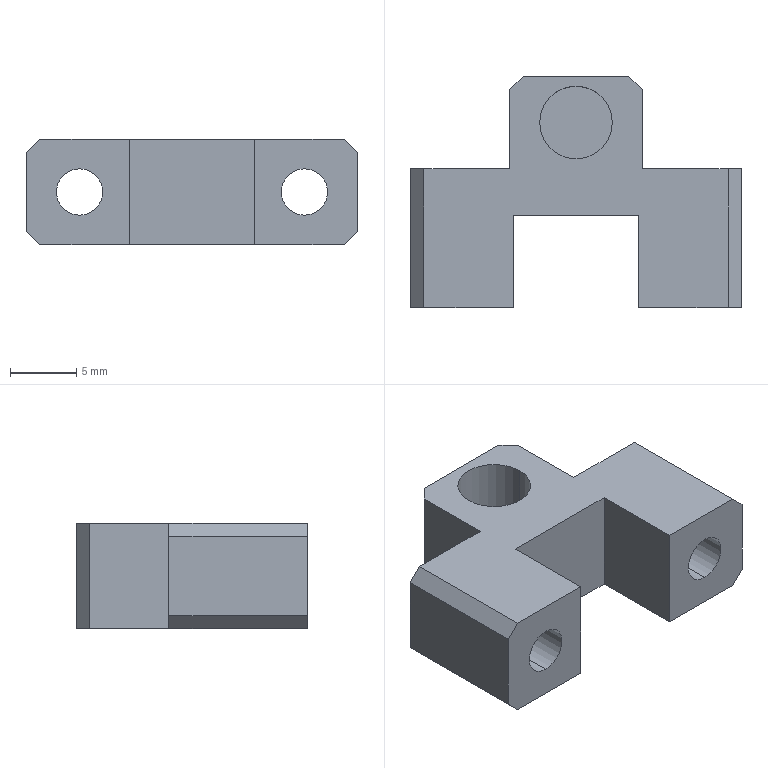Part | SolidWorks | features ICE 3, Chamfer 1, Extrusion 1, HoleWzd 1 | 1 solid | 27 faces | box 25 x 17.5 x 8 mm | volume 1778 mm3 | plane 21 | cylinder 6 | commonest cylinder face diameters 3.5 x4 5.5 x2
STEP:
#1=CARTESIAN_POINT('',(-8.5,-8.75,2.25));
#2=VERTEX_POINT('',#1);
#3=CARTESIAN_POINT('',(-8.5,-8.75,5.75));
#4=VERTEX_POINT('',#3);
#5=CARTESIAN_POINT('',(-8.5,-8.75,4.));
#6=DIRECTION('',(0.,1.,0.));
#7=DIRECTION('',(0.,0.,1.));
#8=AXIS2_PLACEMENT_3D('',#5,#6,#7);
#9=CIRCLE('',#8,1.75);
#10=EDGE_CURVE('',#2,#4,#9,.T.);
#11=ORIENTED_EDGE('',*,*,#10,.F.);
#12=CARTESIAN_POINT('',(-8.5,1.75,2.25));
#13=VERTEX_POINT('',#12);
#14=CARTESIAN_POINT('',(-8.5,1.75,2.25));
#15=DIRECTION('',(0.,1.,0.));
#16=VECTOR('',#15,1000.);
#17=LINE('',#14,#16);
#18=EDGE_CURVE('',#2,#13,#17,.T.);
#19=ORIENTED_EDGE('',*,*,#18,.T.);
#20=CARTESIAN_POINT('',(-8.5,1.75,5.75));
#21=VERTEX_POINT('',#20);
#22=CARTESIAN_POINT('',(-8.5,1.75,4.));
#23=DIRECTION('',(0.,1.,0.));
#24=DIRECTION('',(0.,0.,1.));
#25=AXIS2_PLACEMENT_3D('',#22,#23,#24);
#26=CIRCLE('',#25,1.75);
#27=EDGE_CURVE('',#13,#21,#26,.T.);
#28=ORIENTED_EDGE('',*,*,#27,.T.);
#29=CARTESIAN_POINT('',(-8.5,1.75,5.75));
#30=DIRECTION('',(0.,1.,0.));
#31=VECTOR('',#30,1000.);
#32=LINE('',#29,#31);
#33=EDGE_CURVE('',#4,#21,#32,.T.);
#34=ORIENTED_EDGE('',*,*,#33,.F.);
#35=EDGE_LOOP('',(#11,#19,#28,#34));
#36=FACE_OUTER_BOUND('',#35,.T.);
#37=CARTESIAN_POINT('',(-8.5,1.75,4.));
#38=DIRECTION('',(0.,1.,0.));
#39=DIRECTION('',(0.,0.,1.));
#40=AXIS2_PLACEMENT_3D('',#37,#38,#39);
#41=CYLINDRICAL_SURFACE('',#40,1.75);
#42=ADVANCED_FACE('',(#36),#41,.F.);
#43=CARTESIAN_POINT('',(8.5,-8.75,2.25));
#44=VERTEX_POINT('',#43);
#45=CARTESIAN_POINT('',(8.5,-8.75,5.75));
#46=VERTEX_POINT('',#45);
#47=CARTESIAN_POINT('',(8.5,-8.75,4.));
#48=DIRECTION('',(0.,1.,0.));
#49=DIRECTION('',(0.,0.,1.));
#50=AXIS2_PLACEMENT_3D('',#47,#48,#49);
#51=CIRCLE('',#50,1.75);
#52=EDGE_CURVE('',#44,#46,#51,.T.);
#53=ORIENTED_EDGE('',*,*,#52,.F.);
#54=CARTESIAN_POINT('',(8.5,1.75,2.25));
#55=VERTEX_POINT('',#54);
#56=CARTESIAN_POINT('',(8.5,1.75,2.25));
#57=DIRECTION('',(0.,1.,0.));
#58=VECTOR('',#57,1000.);
#59=LINE('',#56,#58);
#60=EDGE_CURVE('',#44,#55,#59,.T.);
#61=ORIENTED_EDGE('',*,*,#60,.T.);
#62=CARTESIAN_POINT('',(8.5,1.75,5.75));
#63=VERTEX_POINT('',#62);
#64=CARTESIAN_POINT('',(8.5,1.75,4.));
#65=DIRECTION('',(0.,1.,0.));
#66=DIRECTION('',(0.,0.,1.));
#67=AXIS2_PLACEMENT_3D('',#64,#65,#66);
#68=CIRCLE('',#67,1.75);
#69=EDGE_CURVE('',#55,#63,#68,.T.);
#70=ORIENTED_EDGE('',*,*,#69,.T.);
#71=CARTESIAN_POINT('',(8.5,1.75,5.75));
#72=DIRECTION('',(0.,1.,0.));
#73=VECTOR('',#72,1000.);
#74=LINE('',#71,#73);
#75=EDGE_CURVE('',#46,#63,#74,.T.);
#76=ORIENTED_EDGE('',*,*,#75,.F.);
#77=EDGE_LOOP('',(#53,#61,#70,#76));
#78=FACE_OUTER_BOUND('',#77,.T.);
#79=CARTESIAN_POINT('',(8.5,1.75,4.));
#80=DIRECTION('',(0.,1.,0.));
#81=DIRECTION('',(0.,0.,1.));
#82=AXIS2_PLACEMENT_3D('',#79,#80,#81);
#83=CYLINDRICAL_SURFACE('',#82,1.75);
#84=ADVANCED_FACE('',(#78),#83,.F.);
#85=CARTESIAN_POINT('',(-2.75,5.25,3.));
#86=VERTEX_POINT('',#85);
#87=CARTESIAN_POINT('',(2.75,5.25,3.));
#88=VERTEX_POINT('',#87);
#89=CARTESIAN_POINT('',(0.,5.25,3.));
#90=DIRECTION('',(0.,0.,1.));
#91=DIRECTION('',(1.,0.,0.));
#92=AXIS2_PLACEMENT_3D('',#89,#90,#91);
#93=CIRCLE('',#92,2.75);
#94=EDGE_CURVE('',#86,#88,#93,.T.);
#95=ORIENTED_EDGE('',*,*,#94,.F.);
#96=CARTESIAN_POINT('',(-2.75,5.25,8.));
#97=VERTEX_POINT('',#96);
#98=CARTESIAN_POINT('',(-2.75,5.25,3.));
#99=DIRECTION('',(0.,0.,1.));
#100=VECTOR('',#99,1000.);
#101=LINE('',#98,#100);
#102=EDGE_CURVE('',#86,#97,#101,.T.);
#103=ORIENTED_EDGE('',*,*,#102,.T.);
#104=CARTESIAN_POINT('',(2.75,5.25,8.));
#105=VERTEX_POINT('',#104);
#106=CARTESIAN_POINT('',(0.,5.25,8.));
#107=DIRECTION('',(0.,0.,1.));
#108=DIRECTION('',(1.,0.,0.));
#109=AXIS2_PLACEMENT_3D('',#106,#107,#108);
#110=CIRCLE('',#109,2.75);
#111=EDGE_CURVE('',#97,#105,#110,.T.);
#112=ORIENTED_EDGE('',*,*,#111,.T.);
#113=CARTESIAN_POINT('',(2.75,5.25,3.));
#114=DIRECTION('',(0.,0.,1.));
#115=VECTOR('',#114,1000.);
#116=LINE('',#113,#115);
#117=EDGE_CURVE('',#88,#105,#116,.T.);
#118=ORIENTED_EDGE('',*,*,#117,.F.);
#119=EDGE_LOOP('',(#95,#103,#112,#118));
#120=FACE_OUTER_BOUND('',#119,.T.);
#121=CARTESIAN_POINT('',(0.,5.25,3.));
#122=DIRECTION('',(0.,0.,1.));
#123=DIRECTION('',(1.,0.,0.));
#124=AXIS2_PLACEMENT_3D('',#121,#122,#123);
#125=CYLINDRICAL_SURFACE('',#124,2.75);
#126=ADVANCED_FACE('',(#120),#125,.F.);
#127=CARTESIAN_POINT('',(8.5,-8.75,4.));
#128=DIRECTION('',(0.,1.,0.));
#129=DIRECTION('',(0.,0.,1.));
#130=AXIS2_PLACEMENT_3D('',#127,#128,#129);
#131=CIRCLE('',#130,1.75);
#132=EDGE_CURVE('',#46,#44,#131,.T.);
#133=ORIENTED_EDGE('',*,*,#132,.T.);
#134=ORIENTED_EDGE('',*,*,#52,.T.);
#135=EDGE_LOOP('',(#133,#134));
#136=FACE_BOUND('',#135,.T.);
#137=CARTESIAN_POINT('',(4.75,-8.75,0.));
#138=VERTEX_POINT('',#137);
#139=CARTESIAN_POINT('',(11.5,-8.75,0.));
#140=VERTEX_POINT('',#139);
#141=CARTESIAN_POINT('',(-12.5,-8.75,0.));
#142=DIRECTION('',(1.,0.,0.));
#143=VECTOR('',#142,1000.);
#144=LINE('',#141,#143);
#145=EDGE_CURVE('',#138,#140,#144,.T.);
#146=ORIENTED_EDGE('',*,*,#145,.T.);
#147=CARTESIAN_POINT('',(12.5,-8.75,1.));
#148=VERTEX_POINT('',#147);
#149=CARTESIAN_POINT('',(12.5,-8.75,1.));
#150=DIRECTION('',(0.7071,0.,0.7071));
#151=VECTOR('',#150,1000.);
#152=LINE('',#149,#151);
#153=EDGE_CURVE('',#140,#148,#152,.T.);
#154=ORIENTED_EDGE('',*,*,#153,.T.);
#155=CARTESIAN_POINT('',(12.5,-8.75,7.));
#156=VERTEX_POINT('',#155);
#157=CARTESIAN_POINT('',(12.5,-8.75,8.));
#158=DIRECTION('',(0.,0.,-1.));
#159=VECTOR('',#158,1000.);
#160=LINE('',#157,#159);
#161=EDGE_CURVE('',#156,#148,#160,.T.);
#162=ORIENTED_EDGE('',*,*,#161,.F.);
#163=CARTESIAN_POINT('',(11.5,-8.75,8.));
#164=VERTEX_POINT('',#163);
#165=CARTESIAN_POINT('',(11.5,-8.75,8.));
#166=DIRECTION('',(-0.7071,0.,0.7071));
#167=VECTOR('',#166,1000.);
#168=LINE('',#165,#167);
#169=EDGE_CURVE('',#156,#164,#168,.T.);
#170=ORIENTED_EDGE('',*,*,#169,.T.);
#171=CARTESIAN_POINT('',(4.75,-8.75,8.));
#172=VERTEX_POINT('',#171);
#173=CARTESIAN_POINT('',(-12.5,-8.75,8.));
#174=DIRECTION('',(1.,0.,0.));
#175=VECTOR('',#174,1000.);
#176=LINE('',#173,#175);
#177=EDGE_CURVE('',#172,#164,#176,.T.);
#178=ORIENTED_EDGE('',*,*,#177,.F.);
#179=CARTESIAN_POINT('',(4.75,-8.75,0.));
#180=DIRECTION('',(0.,0.,1.));
#181=VECTOR('',#180,1000.);
#182=LINE('',#179,#181);
#183=EDGE_CURVE('',#138,#172,#182,.T.);
#184=ORIENTED_EDGE('',*,*,#183,.F.);
#185=EDGE_LOOP('',(#146,#154,#162,#170,#178,#184));
#186=FACE_OUTER_BOUND('',#185,.T.);
#187=CARTESIAN_POINT('',(-12.5,-8.75,8.));
#188=DIRECTION('',(0.,1.,0.));
#189=DIRECTION('',(0.,0.,1.));
#190=AXIS2_PLACEMENT_3D('',#187,#188,#189);
#191=PLANE('',#190);
#192=ADVANCED_FACE('',(#136,#186),#191,.F.);
#193=ORIENTED_EDGE('',*,*,#161,.T.);
#194=CARTESIAN_POINT('',(12.5,1.75,1.));
#195=VERTEX_POINT('',#194);
#196=CARTESIAN_POINT('',(12.5,1.75,1.));
#197=DIRECTION('',(0.,1.,0.));
#198=VECTOR('',#197,1000.);
#199=LINE('',#196,#198);
#200=EDGE_CURVE('',#148,#195,#199,.T.);
#201=ORIENTED_EDGE('',*,*,#200,.T.);
#202=CARTESIAN_POINT('',(12.5,1.75,7.));
#203=VERTEX_POINT('',#202);
#204=CARTESIAN_POINT('',(12.5,1.75,0.));
#205=DIRECTION('',(0.,0.,1.));
#206=VECTOR('',#205,1000.);
#207=LINE('',#204,#206);
#208=EDGE_CURVE('',#195,#203,#207,.T.);
#209=ORIENTED_EDGE('',*,*,#208,.T.);
#210=CARTESIAN_POINT('',(12.5,-8.75,7.));
#211=DIRECTION('',(0.,-1.,0.));
#212=VECTOR('',#211,1000.);
#213=LINE('',#210,#212);
#214=EDGE_CURVE('',#203,#156,#213,.T.);
#215=ORIENTED_EDGE('',*,*,#214,.T.);
#216=EDGE_LOOP('',(#193,#201,#209,#215));
#217=FACE_OUTER_BOUND('',#216,.T.);
#218=CARTESIAN_POINT('',(12.5,-8.75,8.));
#219=DIRECTION('',(-1.,0.,0.));
#220=DIRECTION('',(0.,0.,1.));
#221=AXIS2_PLACEMENT_3D('',#218,#219,#220);
#222=PLANE('',#221);
#223=ADVANCED_FACE('',(#217),#222,.F.);
#224=CARTESIAN_POINT('',(4.,8.75,0.));
#225=VERTEX_POINT('',#224);
#226=CARTESIAN_POINT('',(-4.,8.75,0.));
#227=VERTEX_POINT('',#226);
#228=CARTESIAN_POINT('',(-12.5,8.75,0.));
#229=DIRECTION('',(-1.,0.,0.));
#230=VECTOR('',#229,1000.);
#231=LINE('',#228,#230);
#232=EDGE_CURVE('',#225,#227,#231,.T.);
#233=ORIENTED_EDGE('',*,*,#232,.T.);
#234=CARTESIAN_POINT('',(-4.,8.75,8.));
#235=VERTEX_POINT('',#234);
#236=CARTESIAN_POINT('',(-4.,8.75,8.));
#237=DIRECTION('',(0.,0.,1.));
#238=VECTOR('',#237,1000.);
#239=LINE('',#236,#238);
#240=EDGE_CURVE('',#227,#235,#239,.T.);
#241=ORIENTED_EDGE('',*,*,#240,.T.);
#242=CARTESIAN_POINT('',(4.,8.75,8.));
#243=VERTEX_POINT('',#242);
#244=CARTESIAN_POINT('',(-12.5,8.75,8.));
#245=DIRECTION('',(-1.,0.,0.));
#246=VECTOR('',#245,1000.);
#247=LINE('',#244,#246);
#248=EDGE_CURVE('',#243,#235,#247,.T.);
#249=ORIENTED_EDGE('',*,*,#248,.F.);
#250=CARTESIAN_POINT('',(4.,8.75,8.));
#251=DIRECTION('',(0.,0.,-1.));
#252=VECTOR('',#251,1000.);
#253=LINE('',#250,#252);
#254=EDGE_CURVE('',#243,#225,#253,.T.);
#255=ORIENTED_EDGE('',*,*,#254,.T.);
#256=EDGE_LOOP('',(#233,#241,#249,#255));
#257=FACE_OUTER_BOUND('',#256,.T.);
#258=CARTESIAN_POINT('',(-12.5,8.75,8.));
#259=DIRECTION('',(0.,-1.,0.));
#260=DIRECTION('',(0.,0.,-1.));
#261=AXIS2_PLACEMENT_3D('',#258,#259,#260);
#262=PLANE('',#261);
#263=ADVANCED_FACE('',(#257),#262,.F.);
#264=CARTESIAN_POINT('',(-12.5,1.75,1.));
#265=VERTEX_POINT('',#264);
#266=CARTESIAN_POINT('',(-12.5,1.75,7.));
#267=VERTEX_POINT('',#266);
#268=CARTESIAN_POINT('',(-12.5,1.75,0.));
#269=DIRECTION('',(0.,0.,1.));
#270=VECTOR('',#269,1000.);
#271=LINE('',#268,#270);
#272=EDGE_CURVE('',#265,#267,#271,.T.);
#273=ORIENTED_EDGE('',*,*,#272,.F.);
#274=CARTESIAN_POINT('',(-12.5,-8.75,1.));
#275=VERTEX_POINT('',#274);
#276=CARTESIAN_POINT('',(-12.5,-8.75,1.));
#277=DIRECTION('',(0.,-1.,0.));
#278=VECTOR('',#277,1000.);
#279=LINE('',#276,#278);
#280=EDGE_CURVE('',#265,#275,#279,.T.);
#281=ORIENTED_EDGE('',*,*,#280,.T.);
#282=CARTESIAN_POINT('',(-12.5,-8.75,7.));
#283=VERTEX_POINT('',#282);
#284=CARTESIAN_POINT('',(-12.5,-8.75,8.));
#285=DIRECTION('',(0.,0.,-1.));
#286=VECTOR('',#285,1000.);
#287=LINE('',#284,#286);
#288=EDGE_CURVE('',#283,#275,#287,.T.);
#289=ORIENTED_EDGE('',*,*,#288,.F.);
#290=CARTESIAN_POINT('',(-12.5,-8.75,7.));
#291=DIRECTION('',(0.,1.,0.));
#292=VECTOR('',#291,1000.);
#293=LINE('',#290,#292);
#294=EDGE_CURVE('',#283,#267,#293,.T.);
#295=ORIENTED_EDGE('',*,*,#294,.T.);
#296=EDGE_LOOP('',(#273,#281,#289,#295));
#297=FACE_OUTER_BOUND('',#296,.T.);
#298=CARTESIAN_POINT('',(-12.5,-8.75,8.));
#299=DIRECTION('',(1.,0.,0.));
#300=DIRECTION('',(0.,0.,-1.));
#301=AXIS2_PLACEMENT_3D('',#298,#299,#300);
#302=PLANE('',#301);
#303=ADVANCED_FACE('',(#297),#302,.F.);
#304=CARTESIAN_POINT('',(-8.5,-8.75,4.));
#305=DIRECTION('',(0.,1.,0.));
#306=DIRECTION('',(0.,0.,1.));
#307=AXIS2_PLACEMENT_3D('',#304,#305,#306);
#308=CIRCLE('',#307,1.75);
#309=EDGE_CURVE('',#4,#2,#308,.T.);
#310=ORIENTED_EDGE('',*,*,#309,.T.);
#311=ORIENTED_EDGE('',*,*,#10,.T.);
#312=EDGE_LOOP('',(#310,#311));
#313=FACE_BOUND('',#312,.T.);
#314=ORIENTED_EDGE('',*,*,#288,.T.);
#315=CARTESIAN_POINT('',(-11.5,-8.75,0.));
#316=VERTEX_POINT('',#315);
#317=CARTESIAN_POINT('',(-12.5,-8.75,1.));
#318=DIRECTION('',(0.7071,0.,-0.7071));
#319=VECTOR('',#318,1000.);
#320=LINE('',#317,#319);
#321=EDGE_CURVE('',#275,#316,#320,.T.);
#322=ORIENTED_EDGE('',*,*,#321,.T.);
#323=CARTESIAN_POINT('',(-4.75,-8.75,0.));
#324=VERTEX_POINT('',#323);
#325=CARTESIAN_POINT('',(-12.5,-8.75,0.));
#326=DIRECTION('',(1.,0.,0.));
#327=VECTOR('',#326,1000.);
#328=LINE('',#325,#327);
#329=EDGE_CURVE('',#316,#324,#328,.T.);
#330=ORIENTED_EDGE('',*,*,#329,.T.);
#331=CARTESIAN_POINT('',(-4.75,-8.75,8.));
#332=VERTEX_POINT('',#331);
#333=CARTESIAN_POINT('',(-4.75,-8.75,0.));
#334=DIRECTION('',(0.,0.,1.));
#335=VECTOR('',#334,1000.);
#336=LINE('',#333,#335);
#337=EDGE_CURVE('',#324,#332,#336,.T.);
#338=ORIENTED_EDGE('',*,*,#337,.T.);
#339=CARTESIAN_POINT('',(-11.5,-8.75,8.));
#340=VERTEX_POINT('',#339);
#341=CARTESIAN_POINT('',(-12.5,-8.75,8.));
#342=DIRECTION('',(1.,0.,0.));
#343=VECTOR('',#342,1000.);
#344=LINE('',#341,#343);
#345=EDGE_CURVE('',#340,#332,#344,.T.);
#346=ORIENTED_EDGE('',*,*,#345,.F.);
#347=CARTESIAN_POINT('',(-11.5,-8.75,8.));
#348=DIRECTION('',(-0.7071,0.,-0.7071));
#349=VECTOR('',#348,1000.);
#350=LINE('',#347,#349);
#351=EDGE_CURVE('',#340,#283,#350,.T.);
#352=ORIENTED_EDGE('',*,*,#351,.T.);
#353=EDGE_LOOP('',(#314,#322,#330,#338,#346,#352));
#354=FACE_OUTER_BOUND('',#353,.T.);
#355=CARTESIAN_POINT('',(-12.5,-8.75,8.));
#356=DIRECTION('',(0.,1.,0.));
#357=DIRECTION('',(0.,0.,1.));
#358=AXIS2_PLACEMENT_3D('',#355,#356,#357);
#359=PLANE('',#358);
#360=ADVANCED_FACE('',(#313,#354),#359,.F.);
#361=CARTESIAN_POINT('',(0.,5.25,8.));
#362=DIRECTION('',(0.,0.,1.));
#363=DIRECTION('',(1.,0.,0.));
#364=AXIS2_PLACEMENT_3D('',#361,#362,#363);
#365=CIRCLE('',#364,2.75);
#366=EDGE_CURVE('',#105,#97,#365,.T.);
#367=ORIENTED_EDGE('',*,*,#366,.F.);
#368=ORIENTED_EDGE('',*,*,#111,.F.);
#369=EDGE_LOOP('',(#367,#368));
#370=FACE_BOUND('',#369,.T.);
#371=ORIENTED_EDGE('',*,*,#248,.T.);
#372=CARTESIAN_POINT('',(-5.,7.75,8.));
#373=VERTEX_POINT('',#372);
#374=CARTESIAN_POINT('',(-4.,8.75,8.));
#375=DIRECTION('',(-0.7071,-0.7071,0.));
#376=VECTOR('',#375,1000.);
#377=LINE('',#374,#376);
#378=EDGE_CURVE('',#235,#373,#377,.T.);
#379=ORIENTED_EDGE('',*,*,#378,.T.);
#380=CARTESIAN_POINT('',(-5.,1.75,8.));
#381=VERTEX_POINT('',#380);
#382=CARTESIAN_POINT('',(-5.,8.75,8.));
#383=DIRECTION('',(0.,1.,0.));
#384=VECTOR('',#383,1000.);
#385=LINE('',#382,#384);
#386=EDGE_CURVE('',#381,#373,#385,.T.);
#387=ORIENTED_EDGE('',*,*,#386,.F.);
#388=CARTESIAN_POINT('',(-11.5,1.75,8.));
#389=VERTEX_POINT('',#388);
#390=CARTESIAN_POINT('',(-12.5,1.75,8.));
#391=DIRECTION('',(1.,0.,0.));
#392=VECTOR('',#391,1000.);
#393=LINE('',#390,#392);
#394=EDGE_CURVE('',#389,#381,#393,.T.);
#395=ORIENTED_EDGE('',*,*,#394,.F.);
#396=CARTESIAN_POINT('',(-11.5,0.,8.));
#397=DIRECTION('',(0.,-1.,0.));
#398=VECTOR('',#397,1000.);
#399=LINE('',#396,#398);
#400=EDGE_CURVE('',#389,#340,#399,.T.);
#401=ORIENTED_EDGE('',*,*,#400,.T.);
#402=ORIENTED_EDGE('',*,*,#345,.T.);
#403=CARTESIAN_POINT('',(-4.75,-1.75,8.));
#404=VERTEX_POINT('',#403);
#405=CARTESIAN_POINT('',(-4.75,-1.75,8.));
#406=DIRECTION('',(0.,-1.,0.));
#407=VECTOR('',#406,1000.);
#408=LINE('',#405,#407);
#409=EDGE_CURVE('',#404,#332,#408,.T.);
#410=ORIENTED_EDGE('',*,*,#409,.F.);
#411=CARTESIAN_POINT('',(4.75,-1.75,8.));
#412=VERTEX_POINT('',#411);
#413=CARTESIAN_POINT('',(-4.75,-1.75,8.));
#414=DIRECTION('',(-1.,0.,0.));
#415=VECTOR('',#414,1000.);
#416=LINE('',#413,#415);
#417=EDGE_CURVE('',#412,#404,#416,.T.);
#418=ORIENTED_EDGE('',*,*,#417,.F.);
#419=CARTESIAN_POINT('',(4.75,-1.75,8.));
#420=DIRECTION('',(0.,1.,0.));
#421=VECTOR('',#420,1000.);
#422=LINE('',#419,#421);
#423=EDGE_CURVE('',#172,#412,#422,.T.);
#424=ORIENTED_EDGE('',*,*,#423,.F.);
#425=ORIENTED_EDGE('',*,*,#177,.T.);
#426=CARTESIAN_POINT('',(11.5,1.75,8.));
#427=VERTEX_POINT('',#426);
#428=CARTESIAN_POINT('',(11.5,0.,8.));
#429=DIRECTION('',(0.,1.,0.));
#430=VECTOR('',#429,1000.);
#431=LINE('',#428,#430);
#432=EDGE_CURVE('',#164,#427,#431,.T.);
#433=ORIENTED_EDGE('',*,*,#432,.T.);
#434=CARTESIAN_POINT('',(5.,1.75,8.));
#435=VERTEX_POINT('',#434);
#436=CARTESIAN_POINT('',(12.5,1.75,8.));
#437=DIRECTION('',(1.,0.,0.));
#438=VECTOR('',#437,1000.);
#439=LINE('',#436,#438);
#440=EDGE_CURVE('',#435,#427,#439,.T.);
#441=ORIENTED_EDGE('',*,*,#440,.F.);
#442=CARTESIAN_POINT('',(5.,7.75,8.));
#443=VERTEX_POINT('',#442);
#444=CARTESIAN_POINT('',(5.,8.75,8.));
#445=DIRECTION('',(0.,-1.,0.));
#446=VECTOR('',#445,1000.);
#447=LINE('',#444,#446);
#448=EDGE_CURVE('',#443,#435,#447,.T.);
#449=ORIENTED_EDGE('',*,*,#448,.F.);
#450=CARTESIAN_POINT('',(5.,7.75,8.));
#451=DIRECTION('',(-0.7071,0.7071,0.));
#452=VECTOR('',#451,1000.);
#453=LINE('',#450,#452);
#454=EDGE_CURVE('',#443,#243,#453,.T.);
#455=ORIENTED_EDGE('',*,*,#454,.T.);
#456=EDGE_LOOP('',(#371,#379,#387,#395,#401,#402,#410,#418,#424,#425,#433,#441,#449,#455));
#457=FACE_OUTER_BOUND('',#456,.T.);
#458=CARTESIAN_POINT('',(0.,0.,8.));
#459=DIRECTION('',(0.,0.,-1.));
#460=DIRECTION('',(-1.,0.,0.));
#461=AXIS2_PLACEMENT_3D('',#458,#459,#460);
#462=PLANE('',#461);
#463=ADVANCED_FACE('',(#370,#457),#462,.F.);
#464=CARTESIAN_POINT('',(-5.,1.75,0.));
#465=VERTEX_POINT('',#464);
#466=CARTESIAN_POINT('',(-5.,7.75,0.));
#467=VERTEX_POINT('',#466);
#468=CARTESIAN_POINT('',(-5.,8.75,0.));
#469=DIRECTION('',(0.,1.,0.));
#470=VECTOR('',#469,1000.);
#471=LINE('',#468,#470);
#472=EDGE_CURVE('',#465,#467,#471,.T.);
#473=ORIENTED_EDGE('',*,*,#472,.T.);
#474=CARTESIAN_POINT('',(-6.375,6.375,0.));
#475=DIRECTION('',(0.7071,0.7071,0.));
#476=VECTOR('',#475,1000.);
#477=LINE('',#474,#476);
#478=EDGE_CURVE('',#467,#227,#477,.T.);
#479=ORIENTED_EDGE('',*,*,#478,.T.);
#480=ORIENTED_EDGE('',*,*,#232,.F.);
#481=CARTESIAN_POINT('',(5.,7.75,0.));
#482=VERTEX_POINT('',#481);
#483=CARTESIAN_POINT('',(6.375,6.375,0.));
#484=DIRECTION('',(0.7071,-0.7071,0.));
#485=VECTOR('',#484,1000.);
#486=LINE('',#483,#485);
#487=EDGE_CURVE('',#225,#482,#486,.T.);
#488=ORIENTED_EDGE('',*,*,#487,.T.);
#489=CARTESIAN_POINT('',(5.,1.75,0.));
#490=VERTEX_POINT('',#489);
#491=CARTESIAN_POINT('',(5.,8.75,0.));
#492=DIRECTION('',(0.,-1.,0.));
#493=VECTOR('',#492,1000.);
#494=LINE('',#491,#493);
#495=EDGE_CURVE('',#482,#490,#494,.T.);
#496=ORIENTED_EDGE('',*,*,#495,.T.);
#497=CARTESIAN_POINT('',(11.5,1.75,0.));
#498=VERTEX_POINT('',#497);
#499=CARTESIAN_POINT('',(12.5,1.75,0.));
#500=DIRECTION('',(1.,0.,0.));
#501=VECTOR('',#500,1000.);
#502=LINE('',#499,#501);
#503=EDGE_CURVE('',#490,#498,#502,.T.);
#504=ORIENTED_EDGE('',*,*,#503,.T.);
#505=CARTESIAN_POINT('',(11.5,-8.75,0.));
#506=DIRECTION('',(0.,-1.,0.));
#507=VECTOR('',#506,1000.);
#508=LINE('',#505,#507);
#509=EDGE_CURVE('',#498,#140,#508,.T.);
#510=ORIENTED_EDGE('',*,*,#509,.T.);
#511=ORIENTED_EDGE('',*,*,#145,.F.);
#512=CARTESIAN_POINT('',(4.75,-1.75,0.));
#513=VERTEX_POINT('',#512);
#514=CARTESIAN_POINT('',(4.75,-1.75,0.));
#515=DIRECTION('',(0.,1.,0.));
#516=VECTOR('',#515,1000.);
#517=LINE('',#514,#516);
#518=EDGE_CURVE('',#138,#513,#517,.T.);
#519=ORIENTED_EDGE('',*,*,#518,.T.);
#520=CARTESIAN_POINT('',(-4.75,-1.75,0.));
#521=VERTEX_POINT('',#520);
#522=CARTESIAN_POINT('',(-4.75,-1.75,0.));
#523=DIRECTION('',(-1.,0.,0.));
#524=VECTOR('',#523,1000.);
#525=LINE('',#522,#524);
#526=EDGE_CURVE('',#513,#521,#525,.T.);
#527=ORIENTED_EDGE('',*,*,#526,.T.);
#528=CARTESIAN_POINT('',(-4.75,-1.75,0.));
#529=DIRECTION('',(0.,-1.,0.));
#530=VECTOR('',#529,1000.);
#531=LINE('',#528,#530);
#532=EDGE_CURVE('',#521,#324,#531,.T.);
#533=ORIENTED_EDGE('',*,*,#532,.T.);
#534=ORIENTED_EDGE('',*,*,#329,.F.);
#535=CARTESIAN_POINT('',(-11.5,1.75,0.));
#536=VERTEX_POINT('',#535);
#537=CARTESIAN_POINT('',(-11.5,1.75,0.));
#538=DIRECTION('',(0.,1.,0.));
#539=VECTOR('',#538,1000.);
#540=LINE('',#537,#539);
#541=EDGE_CURVE('',#316,#536,#540,.T.);
#542=ORIENTED_EDGE('',*,*,#541,.T.);
#543=CARTESIAN_POINT('',(-12.5,1.75,0.));
#544=DIRECTION('',(1.,0.,0.));
#545=VECTOR('',#544,1000.);
#546=LINE('',#543,#545);
#547=EDGE_CURVE('',#536,#465,#546,.T.);
#548=ORIENTED_EDGE('',*,*,#547,.T.);
#549=EDGE_LOOP('',(#473,#479,#480,#488,#496,#504,#510,#511,#519,#527,#533,#534,#542,#548));
#550=FACE_OUTER_BOUND('',#549,.T.);
#551=CARTESIAN_POINT('',(0.,0.,0.));
#552=DIRECTION('',(0.,0.,-1.));
#553=DIRECTION('',(-1.,0.,0.));
#554=AXIS2_PLACEMENT_3D('',#551,#552,#553);
#555=PLANE('',#554);
#556=ADVANCED_FACE('',(#550),#555,.T.);
#557=CARTESIAN_POINT('',(8.5,1.75,4.));
#558=DIRECTION('',(0.,1.,0.));
#559=DIRECTION('',(0.,0.,1.));
#560=AXIS2_PLACEMENT_3D('',#557,#558,#559);
#561=CIRCLE('',#560,1.75);
#562=EDGE_CURVE('',#63,#55,#561,.T.);
#563=ORIENTED_EDGE('',*,*,#562,.F.);
#564=ORIENTED_EDGE('',*,*,#69,.F.);
#565=EDGE_LOOP('',(#563,#564));
#566=FACE_BOUND('',#565,.T.);
#567=ORIENTED_EDGE('',*,*,#208,.F.);
#568=CARTESIAN_POINT('',(12.5,1.75,1.));
#569=DIRECTION('',(-0.7071,0.,-0.7071));
#570=VECTOR('',#569,1000.);
#571=LINE('',#568,#570);
#572=EDGE_CURVE('',#195,#498,#571,.T.);
#573=ORIENTED_EDGE('',*,*,#572,.T.);
#574=ORIENTED_EDGE('',*,*,#503,.F.);
#575=CARTESIAN_POINT('',(5.,1.75,0.));
#576=DIRECTION('',(0.,0.,1.));
#577=VECTOR('',#576,1000.);
#578=LINE('',#575,#577);
#579=EDGE_CURVE('',#490,#435,#578,.T.);
#580=ORIENTED_EDGE('',*,*,#579,.T.);
#581=ORIENTED_EDGE('',*,*,#440,.T.);
#582=CARTESIAN_POINT('',(11.5,1.75,8.));
#583=DIRECTION('',(0.7071,0.,-0.7071));
#584=VECTOR('',#583,1000.);
#585=LINE('',#582,#584);
#586=EDGE_CURVE('',#427,#203,#585,.T.);
#587=ORIENTED_EDGE('',*,*,#586,.T.);
#588=EDGE_LOOP('',(#567,#573,#574,#580,#581,#587));
#589=FACE_OUTER_BOUND('',#588,.T.);
#590=CARTESIAN_POINT('',(12.5,1.75,0.));
#591=DIRECTION('',(0.,-1.,0.));
#592=DIRECTION('',(0.,0.,-1.));
#593=AXIS2_PLACEMENT_3D('',#590,#591,#592);
#594=PLANE('',#593);
#595=ADVANCED_FACE('',(#566,#589),#594,.F.);
#596=ORIENTED_EDGE('',*,*,#495,.F.);
#597=CARTESIAN_POINT('',(5.,7.75,0.));
#598=DIRECTION('',(0.,0.,1.));
#599=VECTOR('',#598,1000.);
#600=LINE('',#597,#599);
#601=EDGE_CURVE('',#482,#443,#600,.T.);
#602=ORIENTED_EDGE('',*,*,#601,.T.);
#603=ORIENTED_EDGE('',*,*,#448,.T.);
#604=ORIENTED_EDGE('',*,*,#579,.F.);
#605=EDGE_LOOP('',(#596,#602,#603,#604));
#606=FACE_OUTER_BOUND('',#605,.T.);
#607=CARTESIAN_POINT('',(5.,8.75,0.));
#608=DIRECTION('',(-1.,0.,0.));
#609=DIRECTION('',(0.,-1.,0.));
#610=AXIS2_PLACEMENT_3D('',#607,#608,#609);
#611=PLANE('',#610);
#612=ADVANCED_FACE('',(#606),#611,.F.);
#613=ORIENTED_EDGE('',*,*,#386,.T.);
#614=CARTESIAN_POINT('',(-5.,7.75,0.));
#615=DIRECTION('',(0.,0.,-1.));
#616=VECTOR('',#615,1000.);
#617=LINE('',#614,#616);
#618=EDGE_CURVE('',#373,#467,#617,.T.);
#619=ORIENTED_EDGE('',*,*,#618,.T.);
#620=ORIENTED_EDGE('',*,*,#472,.F.);
#621=CARTESIAN_POINT('',(-5.,1.75,0.));
#622=DIRECTION('',(0.,0.,1.));
#623=VECTOR('',#622,1000.);
#624=LINE('',#621,#623);
#625=EDGE_CURVE('',#465,#381,#624,.T.);
#626=ORIENTED_EDGE('',*,*,#625,.T.);
#627=EDGE_LOOP('',(#613,#619,#620,#626));
#628=FACE_OUTER_BOUND('',#627,.T.);
#629=CARTESIAN_POINT('',(-5.,8.75,0.));
#630=DIRECTION('',(1.,0.,0.));
#631=DIRECTION('',(0.,1.,0.));
#632=AXIS2_PLACEMENT_3D('',#629,#630,#631);
#633=PLANE('',#632);
#634=ADVANCED_FACE('',(#628),#633,.F.);
#635=CARTESIAN_POINT('',(-8.5,1.75,4.));
#636=DIRECTION('',(0.,1.,0.));
#637=DIRECTION('',(0.,0.,1.));
#638=AXIS2_PLACEMENT_3D('',#635,#636,#637);
#639=CIRCLE('',#638,1.75);
#640=EDGE_CURVE('',#21,#13,#639,.T.);
#641=ORIENTED_EDGE('',*,*,#640,.F.);
#642=ORIENTED_EDGE('',*,*,#27,.F.);
#643=EDGE_LOOP('',(#641,#642));
#644=FACE_BOUND('',#643,.T.);
#645=ORIENTED_EDGE('',*,*,#547,.F.);
#646=CARTESIAN_POINT('',(-12.5,1.75,1.));
#647=DIRECTION('',(-0.7071,0.,0.7071));
#648=VECTOR('',#647,1000.);
#649=LINE('',#646,#648);
#650=EDGE_CURVE('',#536,#265,#649,.T.);
#651=ORIENTED_EDGE('',*,*,#650,.T.);
#652=ORIENTED_EDGE('',*,*,#272,.T.);
#653=CARTESIAN_POINT('',(-11.5,1.75,8.));
#654=DIRECTION('',(0.7071,0.,0.7071));
#655=VECTOR('',#654,1000.);
#656=LINE('',#653,#655);
#657=EDGE_CURVE('',#267,#389,#656,.T.);
#658=ORIENTED_EDGE('',*,*,#657,.T.);
#659=ORIENTED_EDGE('',*,*,#394,.T.);
#660=ORIENTED_EDGE('',*,*,#625,.F.);
#661=EDGE_LOOP('',(#645,#651,#652,#658,#659,#660));
#662=FACE_OUTER_BOUND('',#661,.T.);
#663=CARTESIAN_POINT('',(-12.5,1.75,0.));
#664=DIRECTION('',(0.,-1.,0.));
#665=DIRECTION('',(0.,0.,-1.));
#666=AXIS2_PLACEMENT_3D('',#663,#664,#665);
#667=PLANE('',#666);
#668=ADVANCED_FACE('',(#644,#662),#667,.F.);
#669=ORIENTED_EDGE('',*,*,#423,.T.);
#670=CARTESIAN_POINT('',(4.75,-1.75,0.));
#671=DIRECTION('',(0.,0.,1.));
#672=VECTOR('',#671,1000.);
#673=LINE('',#670,#672);
#674=EDGE_CURVE('',#513,#412,#673,.T.);
#675=ORIENTED_EDGE('',*,*,#674,.F.);
#676=ORIENTED_EDGE('',*,*,#518,.F.);
#677=ORIENTED_EDGE('',*,*,#183,.T.);
#678=EDGE_LOOP('',(#669,#675,#676,#677));
#679=FACE_OUTER_BOUND('',#678,.T.);
#680=CARTESIAN_POINT('',(4.75,-1.75,0.));
#681=DIRECTION('',(1.,0.,0.));
#682=DIRECTION('',(0.,1.,0.));
#683=AXIS2_PLACEMENT_3D('',#680,#681,#682);
#684=PLANE('',#683);
#685=ADVANCED_FACE('',(#679),#684,.F.);
#686=ORIENTED_EDGE('',*,*,#409,.T.);
#687=ORIENTED_EDGE('',*,*,#337,.F.);
#688=ORIENTED_EDGE('',*,*,#532,.F.);
#689=CARTESIAN_POINT('',(-4.75,-1.75,0.));
#690=DIRECTION('',(0.,0.,1.));
#691=VECTOR('',#690,1000.);
#692=LINE('',#689,#691);
#693=EDGE_CURVE('',#521,#404,#692,.T.);
#694=ORIENTED_EDGE('',*,*,#693,.T.);
#695=EDGE_LOOP('',(#686,#687,#688,#694));
#696=FACE_OUTER_BOUND('',#695,.T.);
#697=CARTESIAN_POINT('',(-4.75,-1.75,0.));
#698=DIRECTION('',(-1.,0.,0.));
#699=DIRECTION('',(0.,-1.,0.));
#700=AXIS2_PLACEMENT_3D('',#697,#698,#699);
#701=PLANE('',#700);
#702=ADVANCED_FACE('',(#696),#701,.F.);
#703=ORIENTED_EDGE('',*,*,#417,.T.);
#704=ORIENTED_EDGE('',*,*,#693,.F.);
#705=ORIENTED_EDGE('',*,*,#526,.F.);
#706=ORIENTED_EDGE('',*,*,#674,.T.);
#707=EDGE_LOOP('',(#703,#704,#705,#706));
#708=FACE_OUTER_BOUND('',#707,.T.);
#709=CARTESIAN_POINT('',(-4.75,-1.75,0.));
#710=DIRECTION('',(0.,1.,0.));
#711=DIRECTION('',(0.,0.,1.));
#712=AXIS2_PLACEMENT_3D('',#709,#710,#711);
#713=PLANE('',#712);
#714=ADVANCED_FACE('',(#708),#713,.F.);
#715=ORIENTED_EDGE('',*,*,#102,.F.);
#716=CARTESIAN_POINT('',(0.,5.25,3.));
#717=DIRECTION('',(0.,0.,1.));
#718=DIRECTION('',(1.,0.,0.));
#719=AXIS2_PLACEMENT_3D('',#716,#717,#718);
#720=CIRCLE('',#719,2.75);
#721=EDGE_CURVE('',#88,#86,#720,.T.);
#722=ORIENTED_EDGE('',*,*,#721,.F.);
#723=ORIENTED_EDGE('',*,*,#117,.T.);
#724=ORIENTED_EDGE('',*,*,#366,.T.);
#725=EDGE_LOOP('',(#715,#722,#723,#724));
#726=FACE_OUTER_BOUND('',#725,.T.);
#727=CARTESIAN_POINT('',(0.,5.25,3.));
#728=DIRECTION('',(0.,0.,1.));
#729=DIRECTION('',(1.,0.,0.));
#730=AXIS2_PLACEMENT_3D('',#727,#728,#729);
#731=CYLINDRICAL_SURFACE('',#730,2.75);
#732=ADVANCED_FACE('',(#726),#731,.F.);
#733=ORIENTED_EDGE('',*,*,#721,.T.);
#734=ORIENTED_EDGE('',*,*,#94,.T.);
#735=EDGE_LOOP('',(#733,#734));
#736=FACE_OUTER_BOUND('',#735,.T.);
#737=CARTESIAN_POINT('',(0.,5.25,3.));
#738=DIRECTION('',(0.,0.,1.));
#739=DIRECTION('',(1.,0.,0.));
#740=AXIS2_PLACEMENT_3D('',#737,#738,#739);
#741=PLANE('',#740);
#742=ADVANCED_FACE('',(#736),#741,.T.);
#743=ORIENTED_EDGE('',*,*,#60,.F.);
#744=ORIENTED_EDGE('',*,*,#132,.F.);
#745=ORIENTED_EDGE('',*,*,#75,.T.);
#746=ORIENTED_EDGE('',*,*,#562,.T.);
#747=EDGE_LOOP('',(#743,#744,#745,#746));
#748=FACE_OUTER_BOUND('',#747,.T.);
#749=CARTESIAN_POINT('',(8.5,1.75,4.));
#750=DIRECTION('',(0.,1.,0.));
#751=DIRECTION('',(0.,0.,1.));
#752=AXIS2_PLACEMENT_3D('',#749,#750,#751);
#753=CYLINDRICAL_SURFACE('',#752,1.75);
#754=ADVANCED_FACE('',(#748),#753,.F.);
#755=ORIENTED_EDGE('',*,*,#18,.F.);
#756=ORIENTED_EDGE('',*,*,#309,.F.);
#757=ORIENTED_EDGE('',*,*,#33,.T.);
#758=ORIENTED_EDGE('',*,*,#640,.T.);
#759=EDGE_LOOP('',(#755,#756,#757,#758));
#760=FACE_OUTER_BOUND('',#759,.T.);
#761=CARTESIAN_POINT('',(-8.5,1.75,4.));
#762=DIRECTION('',(0.,1.,0.));
#763=DIRECTION('',(0.,0.,1.));
#764=AXIS2_PLACEMENT_3D('',#761,#762,#763);
#765=CYLINDRICAL_SURFACE('',#764,1.75);
#766=ADVANCED_FACE('',(#760),#765,.F.);
#767=ORIENTED_EDGE('',*,*,#478,.F.);
#768=ORIENTED_EDGE('',*,*,#618,.F.);
#769=ORIENTED_EDGE('',*,*,#378,.F.);
#770=ORIENTED_EDGE('',*,*,#240,.F.);
#771=EDGE_LOOP('',(#767,#768,#769,#770));
#772=FACE_OUTER_BOUND('',#771,.T.);
#773=CARTESIAN_POINT('',(-4.,8.75,8.));
#774=DIRECTION('',(0.7071,-0.7071,0.));
#775=DIRECTION('',(0.,0.,1.));
#776=AXIS2_PLACEMENT_3D('',#773,#774,#775);
#777=PLANE('',#776);
#778=ADVANCED_FACE('',(#772),#777,.F.);
#779=ORIENTED_EDGE('',*,*,#487,.F.);
#780=ORIENTED_EDGE('',*,*,#254,.F.);
#781=ORIENTED_EDGE('',*,*,#454,.F.);
#782=ORIENTED_EDGE('',*,*,#601,.F.);
#783=EDGE_LOOP('',(#779,#780,#781,#782));
#784=FACE_OUTER_BOUND('',#783,.T.);
#785=CARTESIAN_POINT('',(5.,7.75,0.));
#786=DIRECTION('',(-0.7071,-0.7071,0.));
#787=DIRECTION('',(0.,0.,1.));
#788=AXIS2_PLACEMENT_3D('',#785,#786,#787);
#789=PLANE('',#788);
#790=ADVANCED_FACE('',(#784),#789,.F.);
#791=ORIENTED_EDGE('',*,*,#153,.F.);
#792=ORIENTED_EDGE('',*,*,#509,.F.);
#793=ORIENTED_EDGE('',*,*,#572,.F.);
#794=ORIENTED_EDGE('',*,*,#200,.F.);
#795=EDGE_LOOP('',(#791,#792,#793,#794));
#796=FACE_OUTER_BOUND('',#795,.T.);
#797=CARTESIAN_POINT('',(12.5,-8.75,1.));
#798=DIRECTION('',(0.7071,0.,-0.7071));
#799=DIRECTION('',(0.,-1.,0.));
#800=AXIS2_PLACEMENT_3D('',#797,#798,#799);
#801=PLANE('',#800);
#802=ADVANCED_FACE('',(#796),#801,.T.);
#803=ORIENTED_EDGE('',*,*,#169,.F.);
#804=ORIENTED_EDGE('',*,*,#214,.F.);
#805=ORIENTED_EDGE('',*,*,#586,.F.);
#806=ORIENTED_EDGE('',*,*,#432,.F.);
#807=EDGE_LOOP('',(#803,#804,#805,#806));
#808=FACE_OUTER_BOUND('',#807,.T.);
#809=CARTESIAN_POINT('',(11.5,0.,8.));
#810=DIRECTION('',(-0.7071,0.,-0.7071));
#811=DIRECTION('',(0.,1.,0.));
#812=AXIS2_PLACEMENT_3D('',#809,#810,#811);
#813=PLANE('',#812);
#814=ADVANCED_FACE('',(#808),#813,.F.);
#815=ORIENTED_EDGE('',*,*,#650,.F.);
#816=ORIENTED_EDGE('',*,*,#541,.F.);
#817=ORIENTED_EDGE('',*,*,#321,.F.);
#818=ORIENTED_EDGE('',*,*,#280,.F.);
#819=EDGE_LOOP('',(#815,#816,#817,#818));
#820=FACE_OUTER_BOUND('',#819,.T.);
#821=CARTESIAN_POINT('',(-12.5,-8.75,1.));
#822=DIRECTION('',(-0.7071,0.,-0.7071));
#823=DIRECTION('',(0.,1.,0.));
#824=AXIS2_PLACEMENT_3D('',#821,#822,#823);
#825=PLANE('',#824);
#826=ADVANCED_FACE('',(#820),#825,.T.);
#827=ORIENTED_EDGE('',*,*,#657,.F.);
#828=ORIENTED_EDGE('',*,*,#294,.F.);
#829=ORIENTED_EDGE('',*,*,#351,.F.);
#830=ORIENTED_EDGE('',*,*,#400,.F.);
#831=EDGE_LOOP('',(#827,#828,#829,#830));
#832=FACE_OUTER_BOUND('',#831,.T.);
#833=CARTESIAN_POINT('',(-11.5,0.,8.));
#834=DIRECTION('',(0.7071,0.,-0.7071));
#835=DIRECTION('',(0.,-1.,0.));
#836=AXIS2_PLACEMENT_3D('',#833,#834,#835);
#837=PLANE('',#836);
#838=ADVANCED_FACE('',(#832),#837,.F.);
#839=CLOSED_SHELL('',(#42,#84,#126,#192,#223,#263,#303,#360,#463,#556,#595,#612,#634,#668,#685,#702,#714,#732,#742,#754,#766,#778,#790,#802,#814,#826,#838));
#840=MANIFOLD_SOLID_BREP('',#839);
#841=CARTESIAN_POINT('',(0.,0.,0.));
#842=DIRECTION('',(0.,0.,1.));
#843=DIRECTION('',(1.,0.,0.));
#844=AXIS2_PLACEMENT_3D('',#841,#842,#843);
#845=(LENGTH_UNIT()NAMED_UNIT(*)SI_UNIT(.MILLI.,.METRE.));
#846=UNCERTAINTY_MEASURE_WITH_UNIT(LENGTH_MEASURE(0.00001),#845,'','');
#847=(NAMED_UNIT(*)PLANE_ANGLE_UNIT()SI_UNIT($,.RADIAN.));
#848=(NAMED_UNIT(*)SI_UNIT($,.STERADIAN.)SOLID_ANGLE_UNIT());
#849=(GEOMETRIC_REPRESENTATION_CONTEXT(3)GLOBAL_UNCERTAINTY_ASSIGNED_CONTEXT((#846))GLOBAL_UNIT_ASSIGNED_CONTEXT((#845,#847,#848))REPRESENTATION_CONTEXT('',''));
#850=ADVANCED_BREP_SHAPE_REPRESENTATION('',(#840,#844),#849);